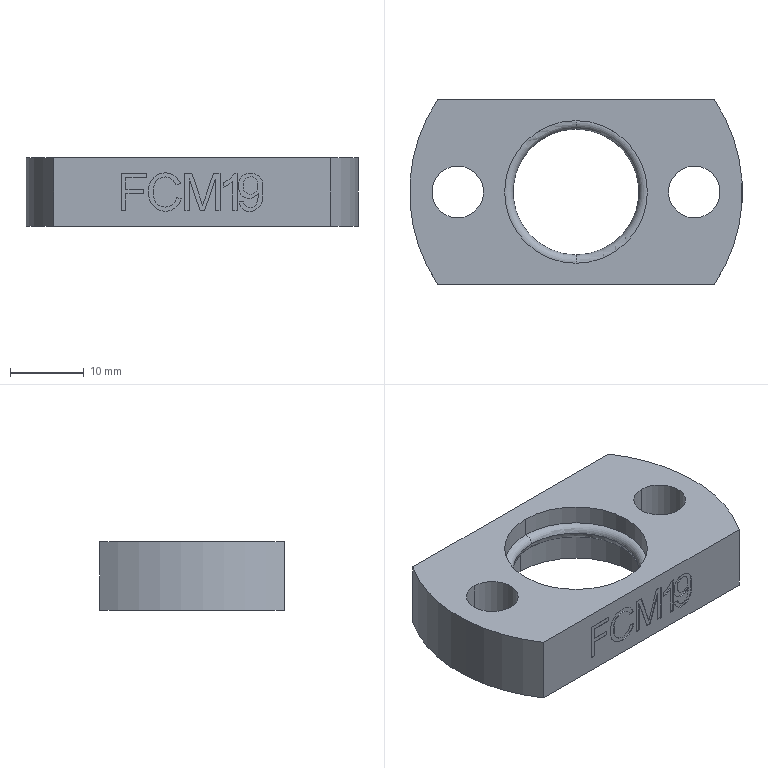Part | STEP file | PN_0054_id498_x_t | 1 solid | 77 faces | box 45 x 25 x 9.2 mm | volume 6185 mm3 | plane 49 | cylinder 24 | spline 2 | torus 2 | commonest cylinder face diameters 7 x4 19.3 x2 21.4 x2 45 x2 1.801 x1 1.989 x1